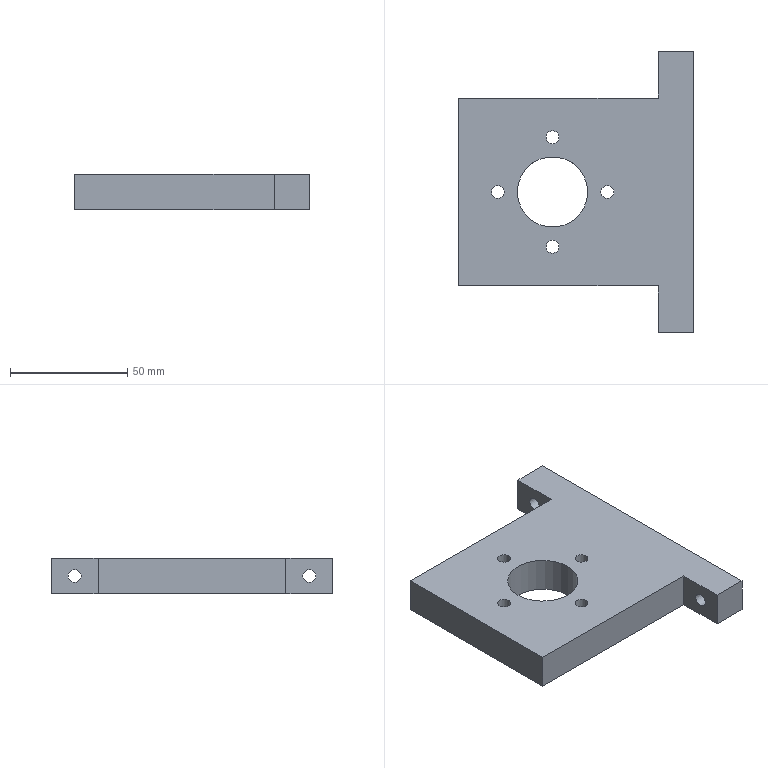Part | NX | features DATUM_CSYS 3, SIMPLE HOLE 2, SKETCH 2, EXTRUDE 1, HOLE PACKAGE 1 | 1 solid | 17 faces | box 100 x 120 x 15 mm | volume 116259 mm3 | plane 10 | cylinder 7 | commonest cylinder face diameters 5.5 x6 30 x1
STEP:
#1=CARTESIAN_POINT('',(-115.,-50.,4.75));
#2=VERTEX_POINT('',#1);
#3=CARTESIAN_POINT('',(-115.,-50.,7.5));
#4=DIRECTION('',(1.,0.,0.));
#5=DIRECTION('',(0.,0.,-1.));
#6=AXIS2_PLACEMENT_3D('',#3,#4,#5);
#7=CIRCLE('',#6,2.75);
#8=EDGE_CURVE('',#2,#2,#7,.T.);
#9=ORIENTED_EDGE('',*,*,#8,.T.);
#10=EDGE_LOOP('',(#9));
#11=FACE_BOUND('',#10,.T.);
#12=CARTESIAN_POINT('',(-115.,-40.,0.));
#13=VERTEX_POINT('',#12);
#14=CARTESIAN_POINT('',(-115.,-60.,0.));
#15=VERTEX_POINT('',#14);
#16=CARTESIAN_POINT('',(-115.,-40.,0.));
#17=DIRECTION('',(0.,-1.,0.));
#18=VECTOR('',#17,1000.);
#19=LINE('',#16,#18);
#20=EDGE_CURVE('',#13,#15,#19,.T.);
#21=ORIENTED_EDGE('',*,*,#20,.T.);
#22=CARTESIAN_POINT('',(-115.,-60.,15.));
#23=VERTEX_POINT('',#22);
#24=CARTESIAN_POINT('',(-115.,-60.,15.));
#25=DIRECTION('',(0.,0.,-1.));
#26=VECTOR('',#25,1000.);
#27=LINE('',#24,#26);
#28=EDGE_CURVE('',#23,#15,#27,.T.);
#29=ORIENTED_EDGE('',*,*,#28,.F.);
#30=CARTESIAN_POINT('',(-115.,-40.,15.));
#31=VERTEX_POINT('',#30);
#32=CARTESIAN_POINT('',(-115.,-40.,15.));
#33=DIRECTION('',(0.,-1.,0.));
#34=VECTOR('',#33,1000.);
#35=LINE('',#32,#34);
#36=EDGE_CURVE('',#31,#23,#35,.T.);
#37=ORIENTED_EDGE('',*,*,#36,.F.);
#38=CARTESIAN_POINT('',(-115.,-40.,15.));
#39=DIRECTION('',(0.,0.,-1.));
#40=VECTOR('',#39,1000.);
#41=LINE('',#38,#40);
#42=EDGE_CURVE('',#31,#13,#41,.T.);
#43=ORIENTED_EDGE('',*,*,#42,.T.);
#44=EDGE_LOOP('',(#21,#29,#37,#43));
#45=FACE_BOUND('',#44,.T.);
#46=CARTESIAN_POINT('',(-115.,-40.,15.));
#47=DIRECTION('',(1.,0.,0.));
#48=DIRECTION('',(0.,0.,-1.));
#49=AXIS2_PLACEMENT_3D('',#46,#47,#48);
#50=PLANE('',#49);
#51=ADVANCED_FACE('',(#11,#45),#50,.F.);
#52=CARTESIAN_POINT('',(-100.,-60.,0.));
#53=VERTEX_POINT('',#52);
#54=CARTESIAN_POINT('',(-115.,-60.,0.));
#55=DIRECTION('',(1.,0.,0.));
#56=VECTOR('',#55,1000.);
#57=LINE('',#54,#56);
#58=EDGE_CURVE('',#15,#53,#57,.T.);
#59=ORIENTED_EDGE('',*,*,#58,.T.);
#60=CARTESIAN_POINT('',(-100.,-60.,15.));
#61=VERTEX_POINT('',#60);
#62=CARTESIAN_POINT('',(-100.,-60.,15.));
#63=DIRECTION('',(0.,0.,-1.));
#64=VECTOR('',#63,1000.);
#65=LINE('',#62,#64);
#66=EDGE_CURVE('',#61,#53,#65,.T.);
#67=ORIENTED_EDGE('',*,*,#66,.F.);
#68=CARTESIAN_POINT('',(-115.,-60.,15.));
#69=DIRECTION('',(1.,0.,0.));
#70=VECTOR('',#69,1000.);
#71=LINE('',#68,#70);
#72=EDGE_CURVE('',#23,#61,#71,.T.);
#73=ORIENTED_EDGE('',*,*,#72,.F.);
#74=ORIENTED_EDGE('',*,*,#28,.T.);
#75=EDGE_LOOP('',(#59,#67,#73,#74));
#76=FACE_BOUND('',#75,.T.);
#77=CARTESIAN_POINT('',(-115.,-60.,15.));
#78=DIRECTION('',(0.,1.,0.));
#79=DIRECTION('',(-1.,0.,0.));
#80=AXIS2_PLACEMENT_3D('',#77,#78,#79);
#81=PLANE('',#80);
#82=ADVANCED_FACE('',(#76),#81,.F.);
#83=CARTESIAN_POINT('',(-100.,50.,10.25));
#84=VERTEX_POINT('',#83);
#85=CARTESIAN_POINT('',(-100.,50.,7.5));
#86=DIRECTION('',(-1.,0.,0.));
#87=DIRECTION('',(0.,0.,1.));
#88=AXIS2_PLACEMENT_3D('',#85,#86,#87);
#89=CIRCLE('',#88,2.75);
#90=EDGE_CURVE('',#84,#84,#89,.T.);
#91=ORIENTED_EDGE('',*,*,#90,.T.);
#92=EDGE_LOOP('',(#91));
#93=FACE_BOUND('',#92,.T.);
#94=CARTESIAN_POINT('',(-100.,-50.,10.25));
#95=VERTEX_POINT('',#94);
#96=CARTESIAN_POINT('',(-100.,-50.,7.5));
#97=DIRECTION('',(-1.,0.,0.));
#98=DIRECTION('',(0.,0.,1.));
#99=AXIS2_PLACEMENT_3D('',#96,#97,#98);
#100=CIRCLE('',#99,2.75);
#101=EDGE_CURVE('',#95,#95,#100,.T.);
#102=ORIENTED_EDGE('',*,*,#101,.T.);
#103=EDGE_LOOP('',(#102));
#104=FACE_BOUND('',#103,.T.);
#105=CARTESIAN_POINT('',(-100.,60.,0.));
#106=VERTEX_POINT('',#105);
#107=CARTESIAN_POINT('',(-100.,-40.,0.));
#108=DIRECTION('',(0.,1.,0.));
#109=VECTOR('',#108,1000.);
#110=LINE('',#107,#109);
#111=EDGE_CURVE('',#53,#106,#110,.T.);
#112=ORIENTED_EDGE('',*,*,#111,.T.);
#113=CARTESIAN_POINT('',(-100.,60.,15.));
#114=VERTEX_POINT('',#113);
#115=CARTESIAN_POINT('',(-100.,60.,15.));
#116=DIRECTION('',(0.,0.,-1.));
#117=VECTOR('',#116,1000.);
#118=LINE('',#115,#117);
#119=EDGE_CURVE('',#114,#106,#118,.T.);
#120=ORIENTED_EDGE('',*,*,#119,.F.);
#121=CARTESIAN_POINT('',(-100.,-60.,15.));
#122=DIRECTION('',(0.,1.,0.));
#123=VECTOR('',#122,1000.);
#124=LINE('',#121,#123);
#125=EDGE_CURVE('',#61,#114,#124,.T.);
#126=ORIENTED_EDGE('',*,*,#125,.F.);
#127=ORIENTED_EDGE('',*,*,#66,.T.);
#128=EDGE_LOOP('',(#112,#120,#126,#127));
#129=FACE_BOUND('',#128,.T.);
#130=CARTESIAN_POINT('',(-100.,-40.,15.));
#131=DIRECTION('',(-1.,0.,0.));
#132=DIRECTION('',(0.,0.,1.));
#133=AXIS2_PLACEMENT_3D('',#130,#131,#132);
#134=PLANE('',#133);
#135=ADVANCED_FACE('',(#93,#104,#129),#134,.F.);
#136=CARTESIAN_POINT('',(-115.,60.,0.));
#137=VERTEX_POINT('',#136);
#138=CARTESIAN_POINT('',(-100.,60.,0.));
#139=DIRECTION('',(-1.,0.,0.));
#140=VECTOR('',#139,1000.);
#141=LINE('',#138,#140);
#142=EDGE_CURVE('',#106,#137,#141,.T.);
#143=ORIENTED_EDGE('',*,*,#142,.T.);
#144=CARTESIAN_POINT('',(-115.,60.,15.));
#145=VERTEX_POINT('',#144);
#146=CARTESIAN_POINT('',(-115.,60.,15.));
#147=DIRECTION('',(0.,0.,-1.));
#148=VECTOR('',#147,1000.);
#149=LINE('',#146,#148);
#150=EDGE_CURVE('',#145,#137,#149,.T.);
#151=ORIENTED_EDGE('',*,*,#150,.F.);
#152=CARTESIAN_POINT('',(-100.,60.,15.));
#153=DIRECTION('',(-1.,0.,0.));
#154=VECTOR('',#153,1000.);
#155=LINE('',#152,#154);
#156=EDGE_CURVE('',#114,#145,#155,.T.);
#157=ORIENTED_EDGE('',*,*,#156,.F.);
#158=ORIENTED_EDGE('',*,*,#119,.T.);
#159=EDGE_LOOP('',(#143,#151,#157,#158));
#160=FACE_BOUND('',#159,.T.);
#161=CARTESIAN_POINT('',(-100.,60.,15.));
#162=DIRECTION('',(0.,-1.,0.));
#163=DIRECTION('',(0.,0.,-1.));
#164=AXIS2_PLACEMENT_3D('',#161,#162,#163);
#165=PLANE('',#164);
#166=ADVANCED_FACE('',(#160),#165,.F.);
#167=CARTESIAN_POINT('',(-115.,50.,4.75));
#168=VERTEX_POINT('',#167);
#169=CARTESIAN_POINT('',(-115.,50.,7.5));
#170=DIRECTION('',(1.,0.,0.));
#171=DIRECTION('',(0.,0.,-1.));
#172=AXIS2_PLACEMENT_3D('',#169,#170,#171);
#173=CIRCLE('',#172,2.75);
#174=EDGE_CURVE('',#168,#168,#173,.T.);
#175=ORIENTED_EDGE('',*,*,#174,.T.);
#176=EDGE_LOOP('',(#175));
#177=FACE_BOUND('',#176,.T.);
#178=CARTESIAN_POINT('',(-115.,40.,0.));
#179=VERTEX_POINT('',#178);
#180=CARTESIAN_POINT('',(-115.,60.,0.));
#181=DIRECTION('',(0.,-1.,0.));
#182=VECTOR('',#181,1000.);
#183=LINE('',#180,#182);
#184=EDGE_CURVE('',#137,#179,#183,.T.);
#185=ORIENTED_EDGE('',*,*,#184,.T.);
#186=CARTESIAN_POINT('',(-115.,40.,15.));
#187=VERTEX_POINT('',#186);
#188=CARTESIAN_POINT('',(-115.,40.,15.));
#189=DIRECTION('',(0.,0.,-1.));
#190=VECTOR('',#189,1000.);
#191=LINE('',#188,#190);
#192=EDGE_CURVE('',#187,#179,#191,.T.);
#193=ORIENTED_EDGE('',*,*,#192,.F.);
#194=CARTESIAN_POINT('',(-115.,60.,15.));
#195=DIRECTION('',(0.,-1.,0.));
#196=VECTOR('',#195,1000.);
#197=LINE('',#194,#196);
#198=EDGE_CURVE('',#145,#187,#197,.T.);
#199=ORIENTED_EDGE('',*,*,#198,.F.);
#200=ORIENTED_EDGE('',*,*,#150,.T.);
#201=EDGE_LOOP('',(#185,#193,#199,#200));
#202=FACE_BOUND('',#201,.T.);
#203=CARTESIAN_POINT('',(-115.,60.,15.));
#204=DIRECTION('',(1.,0.,0.));
#205=DIRECTION('',(0.,0.,-1.));
#206=AXIS2_PLACEMENT_3D('',#203,#204,#205);
#207=PLANE('',#206);
#208=ADVANCED_FACE('',(#177,#202),#207,.F.);
#209=CARTESIAN_POINT('',(-200.,40.,0.));
#210=VERTEX_POINT('',#209);
#211=CARTESIAN_POINT('',(-115.,40.,0.));
#212=DIRECTION('',(-1.,0.,0.));
#213=VECTOR('',#212,1000.);
#214=LINE('',#211,#213);
#215=EDGE_CURVE('',#179,#210,#214,.T.);
#216=ORIENTED_EDGE('',*,*,#215,.T.);
#217=CARTESIAN_POINT('',(-200.,40.,15.));
#218=VERTEX_POINT('',#217);
#219=CARTESIAN_POINT('',(-200.,40.,15.));
#220=DIRECTION('',(0.,0.,-1.));
#221=VECTOR('',#220,1000.);
#222=LINE('',#219,#221);
#223=EDGE_CURVE('',#218,#210,#222,.T.);
#224=ORIENTED_EDGE('',*,*,#223,.F.);
#225=CARTESIAN_POINT('',(-115.,40.,15.));
#226=DIRECTION('',(-1.,0.,0.));
#227=VECTOR('',#226,1000.);
#228=LINE('',#225,#227);
#229=EDGE_CURVE('',#187,#218,#228,.T.);
#230=ORIENTED_EDGE('',*,*,#229,.F.);
#231=ORIENTED_EDGE('',*,*,#192,.T.);
#232=EDGE_LOOP('',(#216,#224,#230,#231));
#233=FACE_BOUND('',#232,.T.);
#234=CARTESIAN_POINT('',(-115.,40.,15.));
#235=DIRECTION('',(0.,-1.,0.));
#236=DIRECTION('',(0.,0.,-1.));
#237=AXIS2_PLACEMENT_3D('',#234,#235,#236);
#238=PLANE('',#237);
#239=ADVANCED_FACE('',(#233),#238,.F.);
#240=CARTESIAN_POINT('',(-200.,-40.,0.));
#241=VERTEX_POINT('',#240);
#242=CARTESIAN_POINT('',(-200.,40.,0.));
#243=DIRECTION('',(0.,-1.,0.));
#244=VECTOR('',#243,1000.);
#245=LINE('',#242,#244);
#246=EDGE_CURVE('',#210,#241,#245,.T.);
#247=ORIENTED_EDGE('',*,*,#246,.T.);
#248=CARTESIAN_POINT('',(-200.,-40.,15.));
#249=VERTEX_POINT('',#248);
#250=CARTESIAN_POINT('',(-200.,-40.,15.));
#251=DIRECTION('',(0.,0.,-1.));
#252=VECTOR('',#251,1000.);
#253=LINE('',#250,#252);
#254=EDGE_CURVE('',#249,#241,#253,.T.);
#255=ORIENTED_EDGE('',*,*,#254,.F.);
#256=CARTESIAN_POINT('',(-200.,40.,15.));
#257=DIRECTION('',(0.,-1.,0.));
#258=VECTOR('',#257,1000.);
#259=LINE('',#256,#258);
#260=EDGE_CURVE('',#218,#249,#259,.T.);
#261=ORIENTED_EDGE('',*,*,#260,.F.);
#262=ORIENTED_EDGE('',*,*,#223,.T.);
#263=EDGE_LOOP('',(#247,#255,#261,#262));
#264=FACE_BOUND('',#263,.T.);
#265=CARTESIAN_POINT('',(-200.,40.,15.));
#266=DIRECTION('',(1.,0.,0.));
#267=DIRECTION('',(0.,0.,-1.));
#268=AXIS2_PLACEMENT_3D('',#265,#266,#267);
#269=PLANE('',#268);
#270=ADVANCED_FACE('',(#264),#269,.F.);
#271=CARTESIAN_POINT('',(-162.75,23.33,15.));
#272=VERTEX_POINT('',#271);
#273=CARTESIAN_POINT('',(-160.,23.33,15.));
#274=DIRECTION('',(0.,0.,1.));
#275=DIRECTION('',(-1.,0.,0.));
#276=AXIS2_PLACEMENT_3D('',#273,#274,#275);
#277=CIRCLE('',#276,2.75);
#278=EDGE_CURVE('',#272,#272,#277,.T.);
#279=ORIENTED_EDGE('',*,*,#278,.T.);
#280=EDGE_LOOP('',(#279));
#281=FACE_BOUND('',#280,.T.);
#282=CARTESIAN_POINT('',(-162.75,23.33,0.));
#283=VERTEX_POINT('',#282);
#284=CARTESIAN_POINT('',(-160.,23.33,0.));
#285=DIRECTION('',(0.,0.,1.));
#286=DIRECTION('',(-1.,0.,0.));
#287=AXIS2_PLACEMENT_3D('',#284,#285,#286);
#288=CIRCLE('',#287,2.75);
#289=EDGE_CURVE('',#283,#283,#288,.T.);
#290=ORIENTED_EDGE('',*,*,#289,.F.);
#291=EDGE_LOOP('',(#290));
#292=FACE_BOUND('',#291,.T.);
#293=CARTESIAN_POINT('',(-160.,23.33,15.));
#294=DIRECTION('',(0.,0.,-1.));
#295=DIRECTION('',(-1.,0.,0.));
#296=AXIS2_PLACEMENT_3D('',#293,#294,#295);
#297=CYLINDRICAL_SURFACE('',#296,2.75);
#298=ADVANCED_FACE('',(#281,#292),#297,.F.);
#299=CARTESIAN_POINT('',(-157.25,-23.33,15.));
#300=VERTEX_POINT('',#299);
#301=CARTESIAN_POINT('',(-160.,-23.33,15.));
#302=DIRECTION('',(0.,0.,1.));
#303=DIRECTION('',(1.,0.,0.));
#304=AXIS2_PLACEMENT_3D('',#301,#302,#303);
#305=CIRCLE('',#304,2.75);
#306=EDGE_CURVE('',#300,#300,#305,.T.);
#307=ORIENTED_EDGE('',*,*,#306,.T.);
#308=EDGE_LOOP('',(#307));
#309=FACE_BOUND('',#308,.T.);
#310=CARTESIAN_POINT('',(-157.25,-23.33,0.));
#311=VERTEX_POINT('',#310);
#312=CARTESIAN_POINT('',(-160.,-23.33,0.));
#313=DIRECTION('',(0.,0.,1.));
#314=DIRECTION('',(1.,0.,0.));
#315=AXIS2_PLACEMENT_3D('',#312,#313,#314);
#316=CIRCLE('',#315,2.75);
#317=EDGE_CURVE('',#311,#311,#316,.T.);
#318=ORIENTED_EDGE('',*,*,#317,.F.);
#319=EDGE_LOOP('',(#318));
#320=FACE_BOUND('',#319,.T.);
#321=CARTESIAN_POINT('',(-160.,-23.33,15.));
#322=DIRECTION('',(0.,0.,-1.));
#323=DIRECTION('',(-1.,0.,0.));
#324=AXIS2_PLACEMENT_3D('',#321,#322,#323);
#325=CYLINDRICAL_SURFACE('',#324,2.75);
#326=ADVANCED_FACE('',(#309,#320),#325,.F.);
#327=CARTESIAN_POINT('',(-145.,0.,15.));
#328=VERTEX_POINT('',#327);
#329=CARTESIAN_POINT('',(-160.,0.,15.));
#330=DIRECTION('',(0.,0.,1.));
#331=DIRECTION('',(1.,0.,0.));
#332=AXIS2_PLACEMENT_3D('',#329,#330,#331);
#333=CIRCLE('',#332,15.);
#334=EDGE_CURVE('',#328,#328,#333,.T.);
#335=ORIENTED_EDGE('',*,*,#334,.T.);
#336=EDGE_LOOP('',(#335));
#337=FACE_BOUND('',#336,.T.);
#338=CARTESIAN_POINT('',(-145.,0.,0.));
#339=VERTEX_POINT('',#338);
#340=CARTESIAN_POINT('',(-160.,0.,0.));
#341=DIRECTION('',(0.,0.,1.));
#342=DIRECTION('',(1.,0.,0.));
#343=AXIS2_PLACEMENT_3D('',#340,#341,#342);
#344=CIRCLE('',#343,15.);
#345=EDGE_CURVE('',#339,#339,#344,.T.);
#346=ORIENTED_EDGE('',*,*,#345,.F.);
#347=EDGE_LOOP('',(#346));
#348=FACE_BOUND('',#347,.T.);
#349=CARTESIAN_POINT('',(-160.,0.,15.));
#350=DIRECTION('',(0.,0.,-1.));
#351=DIRECTION('',(-1.,0.,0.));
#352=AXIS2_PLACEMENT_3D('',#349,#350,#351);
#353=CYLINDRICAL_SURFACE('',#352,15.);
#354=ADVANCED_FACE('',(#337,#348),#353,.F.);
#355=CARTESIAN_POINT('',(-183.33,-2.75,15.));
#356=VERTEX_POINT('',#355);
#357=CARTESIAN_POINT('',(-183.33,0.,15.));
#358=DIRECTION('',(0.,0.,1.));
#359=DIRECTION('',(0.,-1.,0.));
#360=AXIS2_PLACEMENT_3D('',#357,#358,#359);
#361=CIRCLE('',#360,2.75);
#362=EDGE_CURVE('',#356,#356,#361,.T.);
#363=ORIENTED_EDGE('',*,*,#362,.T.);
#364=EDGE_LOOP('',(#363));
#365=FACE_BOUND('',#364,.T.);
#366=CARTESIAN_POINT('',(-183.33,-2.75,0.));
#367=VERTEX_POINT('',#366);
#368=CARTESIAN_POINT('',(-183.33,0.,0.));
#369=DIRECTION('',(0.,0.,1.));
#370=DIRECTION('',(0.,-1.,0.));
#371=AXIS2_PLACEMENT_3D('',#368,#369,#370);
#372=CIRCLE('',#371,2.75);
#373=EDGE_CURVE('',#367,#367,#372,.T.);
#374=ORIENTED_EDGE('',*,*,#373,.F.);
#375=EDGE_LOOP('',(#374));
#376=FACE_BOUND('',#375,.T.);
#377=CARTESIAN_POINT('',(-183.33,0.,15.));
#378=DIRECTION('',(0.,0.,-1.));
#379=DIRECTION('',(-1.,0.,0.));
#380=AXIS2_PLACEMENT_3D('',#377,#378,#379);
#381=CYLINDRICAL_SURFACE('',#380,2.75);
#382=ADVANCED_FACE('',(#365,#376),#381,.F.);
#383=CARTESIAN_POINT('',(-200.,-40.,0.));
#384=DIRECTION('',(1.,0.,0.));
#385=VECTOR('',#384,1000.);
#386=LINE('',#383,#385);
#387=EDGE_CURVE('',#241,#13,#386,.T.);
#388=ORIENTED_EDGE('',*,*,#387,.T.);
#389=ORIENTED_EDGE('',*,*,#42,.F.);
#390=CARTESIAN_POINT('',(-200.,-40.,15.));
#391=DIRECTION('',(1.,0.,0.));
#392=VECTOR('',#391,1000.);
#393=LINE('',#390,#392);
#394=EDGE_CURVE('',#249,#31,#393,.T.);
#395=ORIENTED_EDGE('',*,*,#394,.F.);
#396=ORIENTED_EDGE('',*,*,#254,.T.);
#397=EDGE_LOOP('',(#388,#389,#395,#396));
#398=FACE_BOUND('',#397,.T.);
#399=CARTESIAN_POINT('',(-200.,-40.,15.));
#400=DIRECTION('',(0.,1.,0.));
#401=DIRECTION('',(0.,0.,1.));
#402=AXIS2_PLACEMENT_3D('',#399,#400,#401);
#403=PLANE('',#402);
#404=ADVANCED_FACE('',(#398),#403,.F.);
#405=CARTESIAN_POINT('',(-136.67,2.75,15.));
#406=VERTEX_POINT('',#405);
#407=CARTESIAN_POINT('',(-136.67,0.,15.));
#408=DIRECTION('',(0.,0.,1.));
#409=DIRECTION('',(0.,1.,0.));
#410=AXIS2_PLACEMENT_3D('',#407,#408,#409);
#411=CIRCLE('',#410,2.75);
#412=EDGE_CURVE('',#406,#406,#411,.T.);
#413=ORIENTED_EDGE('',*,*,#412,.T.);
#414=EDGE_LOOP('',(#413));
#415=FACE_BOUND('',#414,.T.);
#416=CARTESIAN_POINT('',(-136.67,2.75,0.));
#417=VERTEX_POINT('',#416);
#418=CARTESIAN_POINT('',(-136.67,0.,0.));
#419=DIRECTION('',(0.,0.,1.));
#420=DIRECTION('',(0.,1.,0.));
#421=AXIS2_PLACEMENT_3D('',#418,#419,#420);
#422=CIRCLE('',#421,2.75);
#423=EDGE_CURVE('',#417,#417,#422,.T.);
#424=ORIENTED_EDGE('',*,*,#423,.F.);
#425=EDGE_LOOP('',(#424));
#426=FACE_BOUND('',#425,.T.);
#427=CARTESIAN_POINT('',(-136.67,0.,15.));
#428=DIRECTION('',(0.,0.,-1.));
#429=DIRECTION('',(-1.,0.,0.));
#430=AXIS2_PLACEMENT_3D('',#427,#428,#429);
#431=CYLINDRICAL_SURFACE('',#430,2.75);
#432=ADVANCED_FACE('',(#415,#426),#431,.F.);
#433=ORIENTED_EDGE('',*,*,#36,.T.);
#434=ORIENTED_EDGE('',*,*,#72,.T.);
#435=ORIENTED_EDGE('',*,*,#125,.T.);
#436=ORIENTED_EDGE('',*,*,#156,.T.);
#437=ORIENTED_EDGE('',*,*,#198,.T.);
#438=ORIENTED_EDGE('',*,*,#229,.T.);
#439=ORIENTED_EDGE('',*,*,#260,.T.);
#440=ORIENTED_EDGE('',*,*,#394,.T.);
#441=EDGE_LOOP('',(#433,#434,#435,#436,#437,#438,#439,#440));
#442=FACE_BOUND('',#441,.T.);
#443=ORIENTED_EDGE('',*,*,#362,.F.);
#444=EDGE_LOOP('',(#443));
#445=FACE_BOUND('',#444,.T.);
#446=ORIENTED_EDGE('',*,*,#334,.F.);
#447=EDGE_LOOP('',(#446));
#448=FACE_BOUND('',#447,.T.);
#449=ORIENTED_EDGE('',*,*,#306,.F.);
#450=EDGE_LOOP('',(#449));
#451=FACE_BOUND('',#450,.T.);
#452=ORIENTED_EDGE('',*,*,#278,.F.);
#453=EDGE_LOOP('',(#452));
#454=FACE_BOUND('',#453,.T.);
#455=ORIENTED_EDGE('',*,*,#412,.F.);
#456=EDGE_LOOP('',(#455));
#457=FACE_BOUND('',#456,.T.);
#458=CARTESIAN_POINT('',(-183.33,0.,15.));
#459=DIRECTION('',(0.,0.,1.));
#460=DIRECTION('',(1.,0.,0.));
#461=AXIS2_PLACEMENT_3D('',#458,#459,#460);
#462=PLANE('',#461);
#463=ADVANCED_FACE('',(#442,#445,#448,#451,#454,#457),#462,.T.);
#464=ORIENTED_EDGE('',*,*,#20,.F.);
#465=ORIENTED_EDGE('',*,*,#387,.F.);
#466=ORIENTED_EDGE('',*,*,#246,.F.);
#467=ORIENTED_EDGE('',*,*,#215,.F.);
#468=ORIENTED_EDGE('',*,*,#184,.F.);
#469=ORIENTED_EDGE('',*,*,#142,.F.);
#470=ORIENTED_EDGE('',*,*,#111,.F.);
#471=ORIENTED_EDGE('',*,*,#58,.F.);
#472=EDGE_LOOP('',(#464,#465,#466,#467,#468,#469,#470,#471));
#473=FACE_BOUND('',#472,.T.);
#474=ORIENTED_EDGE('',*,*,#373,.T.);
#475=EDGE_LOOP('',(#474));
#476=FACE_BOUND('',#475,.T.);
#477=ORIENTED_EDGE('',*,*,#345,.T.);
#478=EDGE_LOOP('',(#477));
#479=FACE_BOUND('',#478,.T.);
#480=ORIENTED_EDGE('',*,*,#317,.T.);
#481=EDGE_LOOP('',(#480));
#482=FACE_BOUND('',#481,.T.);
#483=ORIENTED_EDGE('',*,*,#289,.T.);
#484=EDGE_LOOP('',(#483));
#485=FACE_BOUND('',#484,.T.);
#486=ORIENTED_EDGE('',*,*,#423,.T.);
#487=EDGE_LOOP('',(#486));
#488=FACE_BOUND('',#487,.T.);
#489=CARTESIAN_POINT('',(-183.33,0.,0.));
#490=DIRECTION('',(0.,0.,1.));
#491=DIRECTION('',(1.,0.,0.));
#492=AXIS2_PLACEMENT_3D('',#489,#490,#491);
#493=PLANE('',#492);
#494=ADVANCED_FACE('',(#473,#476,#479,#482,#485,#488),#493,.F.);
#495=ORIENTED_EDGE('',*,*,#8,.F.);
#496=EDGE_LOOP('',(#495));
#497=FACE_BOUND('',#496,.T.);
#498=ORIENTED_EDGE('',*,*,#101,.F.);
#499=EDGE_LOOP('',(#498));
#500=FACE_BOUND('',#499,.T.);
#501=CARTESIAN_POINT('',(-115.,-50.,7.5));
#502=DIRECTION('',(1.,0.,0.));
#503=DIRECTION('',(0.,0.,-1.));
#504=AXIS2_PLACEMENT_3D('',#501,#502,#503);
#505=CYLINDRICAL_SURFACE('',#504,2.75);
#506=ADVANCED_FACE('',(#497,#500),#505,.F.);
#507=ORIENTED_EDGE('',*,*,#174,.F.);
#508=EDGE_LOOP('',(#507));
#509=FACE_BOUND('',#508,.T.);
#510=ORIENTED_EDGE('',*,*,#90,.F.);
#511=EDGE_LOOP('',(#510));
#512=FACE_BOUND('',#511,.T.);
#513=CARTESIAN_POINT('',(-115.,50.,7.5));
#514=DIRECTION('',(1.,0.,0.));
#515=DIRECTION('',(0.,0.,-1.));
#516=AXIS2_PLACEMENT_3D('',#513,#514,#515);
#517=CYLINDRICAL_SURFACE('',#516,2.75);
#518=ADVANCED_FACE('',(#509,#512),#517,.F.);
#519=CLOSED_SHELL('',(#51,#82,#135,#166,#208,#239,#270,#298,#326,#354,#382,#404,#432,#463,#494,#506,#518));
#520=MANIFOLD_SOLID_BREP('',#519);
#521=(LENGTH_UNIT()NAMED_UNIT(*)SI_UNIT(.MILLI.,.METRE.));
#522=UNCERTAINTY_MEASURE_WITH_UNIT(LENGTH_MEASURE(0.00001),#521,'','');
#523=(NAMED_UNIT(*)PLANE_ANGLE_UNIT()SI_UNIT($,.RADIAN.));
#524=(NAMED_UNIT(*)SI_UNIT($,.STERADIAN.)SOLID_ANGLE_UNIT());
#525=(GEOMETRIC_REPRESENTATION_CONTEXT(3)GLOBAL_UNCERTAINTY_ASSIGNED_CONTEXT((#522))GLOBAL_UNIT_ASSIGNED_CONTEXT((#521,#523,#524))REPRESENTATION_CONTEXT('',''));
#526=ADVANCED_BREP_SHAPE_REPRESENTATION('',(#520),#525);